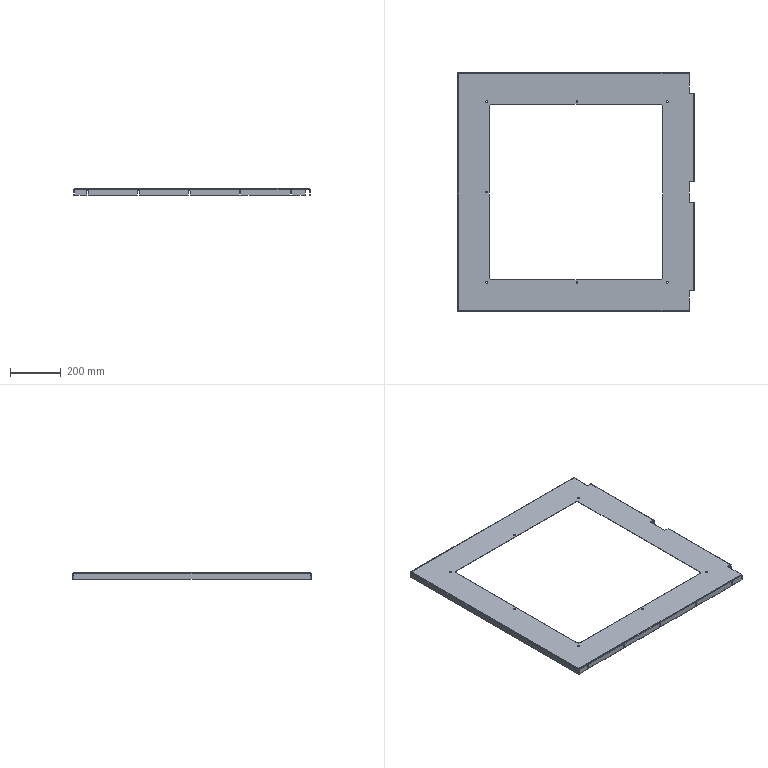Part | STEP file | SynoNew-0304-057 | 1 solid | 107 faces | box 928 x 936 x 25 mm | volume 704183 mm3 | plane 76 | cylinder 31 | commonest cylinder face diameters 6.6 x17 3 x5 6 x5 20 x4